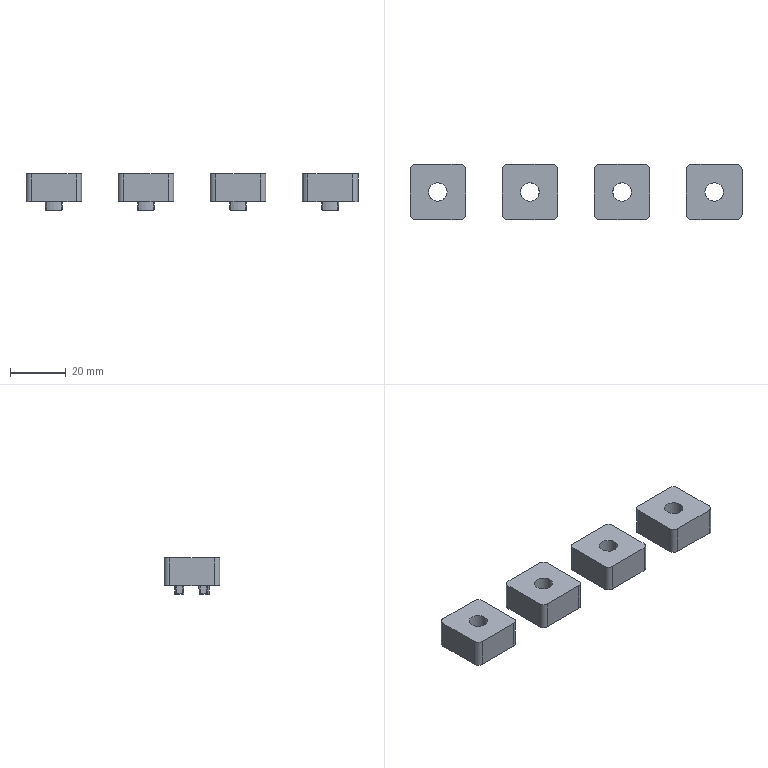NC program | NX | posted with a generic post | part box 118.91 x 19.91 x 13 mm
Lines 3894 to 4008 of 17620:
(ZLEVEL_PROFILE_1 , TOOL : D10JING)
N7780 T14 M6
N7782 G54
N7784 G17 G0 G90 X26.178 Y-16.897 S9500 M3
N7786 G43 Z30. H14
N7788 Z-11.5
N7790 G94 G1 Z-13. F1000.
N7792 G41 X26.144 Y-16.803 D14
N7794 X25.366 Y-15.455
N7796 G3 X24.5 Y-14.955 R1.
N7798 G1 X8.5 F1500.
N7800 G2 X1.545 Y-8. R6.955
N7802 G1 Y8.
N7804 G2 X8.5 Y14.955 R6.955
N7806 G1 X24.5
N7808 G2 X31.455 Y8. R6.955
N7810 G1 Y-8.
N7812 G2 X24.5 Y-14.955 R6.955
N7814 G3 X23.634 Y-15.455 R1.
N7816 G1 X22.768 Y-16.955
N7818 G40
N7820 X22.734 Y-17.049
N7822 Z-11.5
N7824 G0 Z30.
N7826 X59.178 Y-16.897
N7828 Z-11.5
N7830 G1 Z-13. F1000.
N7832 G41 X59.144 Y-16.803
N7834 X58.366 Y-15.455
N7836 G3 X57.5 Y-14.955 R1.
N7838 G1 X41.5 F1500.
N7840 G2 X34.545 Y-8. R6.955
N7842 G1 Y8.
N7844 G2 X41.5 Y14.955 R6.955
N7846 G1 X57.5
N7848 G2 X64.455 Y8. R6.955
N7850 G1 Y-8.
N7852 G2 X57.5 Y-14.955 R6.955
N7854 G3 X56.634 Y-15.455 R1.
N7856 G1 X55.768 Y-16.955
N7858 G40
N7860 X55.734 Y-17.049
N7862 Z-11.5
N7864 G0 Z30.
N7866 X-6.822 Y-16.897
N7868 Z-11.5
N7870 G1 Z-13. F1000.
N7872 G41 X-6.856 Y-16.803
N7874 X-7.634 Y-15.455
N7876 G3 X-8.5 Y-14.955 R1.
N7878 G1 X-24.5 F1500.
N7880 G2 X-31.455 Y-8. R6.955
N7882 G1 Y8.
N7884 G2 X-24.5 Y14.955 R6.955
N7886 G1 X-8.5
N7888 G2 X-1.545 Y8. R6.955
N7890 G1 Y-8.
N7892 G2 X-8.5 Y-14.955 R6.955
N7894 G3 X-9.366 Y-15.455 R1.
N7896 G1 X-10.232 Y-16.955
N7898 G40
N7900 X-10.266 Y-17.049
N7902 Z-11.5
N7904 G0 Z30.
N7906 X-39.822 Y-16.897
N7908 Z-11.5
N7910 G1 Z-13. F1000.
N7912 G41 X-39.856 Y-16.803
N7914 X-40.634 Y-15.455
N7916 G3 X-41.5 Y-14.955 R1.
N7918 G1 X-57.5 F1500.
N7920 G2 X-64.455 Y-8. R6.955
N7922 G1 Y8.
N7924 G2 X-57.5 Y14.955 R6.955
N7926 G1 X-41.5
N7928 G2 X-34.545 Y8. R6.955
N7930 G1 Y-8.
N7932 G2 X-41.5 Y-14.955 R6.955
N7934 G3 X-42.366 Y-15.455 R1.
N7936 G1 X-43.232 Y-16.955
N7938 G40
N7940 X-43.266 Y-17.049
N7942 Z-11.5
N7944 G0 Z30.
N7946 M5
(DRILLING , TOOL : D6A45)
N7948 T01 M6
N7950 G54
N7952 G17 G0 G90 X-49.5 Y0. S5000 M3
N7954 G43 Z30. H1
N7956 G94 G81 G98 Z-1. F250. R3.
N7958 X-16.5
N7960 X16.5
N7962 X49.5
N7964 G80
N7966 G0 X49.5 Y0. Z30.
N7968 M5
(DRILLING_COPY , TOOL : 6.6ZT)
N7970 T16 M6
N7972 G54
N7974 G17 G0 G90 X-49.5 Y0. S2004 M3
N7976 G43 Z30. H16
N7978 G94 G83 G98 Z-16.483 F250. Q2. R3.
N7980 X-16.5
N7982 X16.5
N7984 X49.5
N7986 G80
N7988 G0 X49.5 Y0. Z30.
N7990 M5